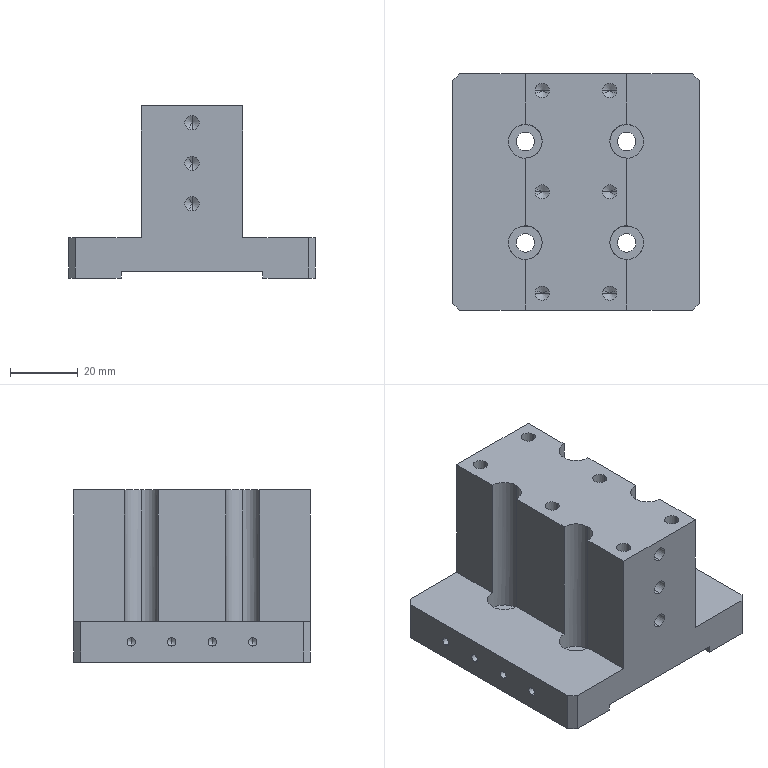Part | STEP file | 06-02KK60模组连接块 | 1 solid | 122 faces | box 73 x 70 x 51 mm | volume 125867 mm3 | cylinder 56 | cone 40 | plane 26 | commonest cylinder face diameters 4.2 x24 2.5 x16 5.5 x8 10 x8